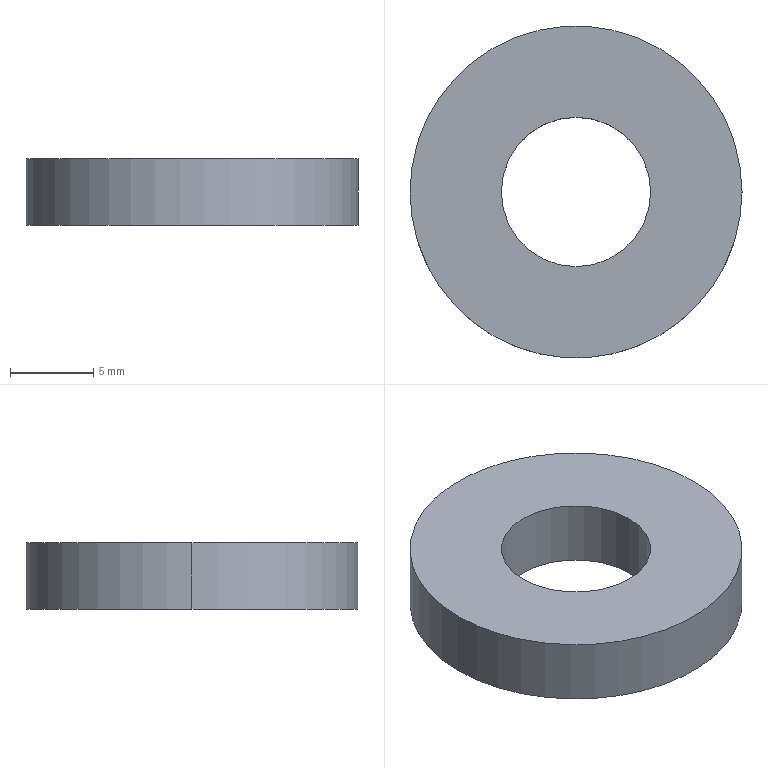Part | SolidWorks | features Extrusion 1 | 1 solid | 6 faces | box 20 x 20 x 4 mm | volume 1002 mm3 | cylinder 4 | plane 2 | commonest cylinder face diameters 9 x2 20 x2
STEP:
#1=CARTESIAN_POINT('',(-4.5,0.,4.));
#2=VERTEX_POINT('',#1);
#3=CARTESIAN_POINT('',(4.5,0.,4.));
#4=VERTEX_POINT('',#3);
#5=CARTESIAN_POINT('',(0.,0.,4.));
#6=DIRECTION('',(0.,0.,1.));
#7=DIRECTION('',(1.,0.,0.));
#8=AXIS2_PLACEMENT_3D('',#5,#6,#7);
#9=CIRCLE('',#8,4.5);
#10=EDGE_CURVE('',#2,#4,#9,.T.);
#11=ORIENTED_EDGE('',*,*,#10,.T.);
#12=CARTESIAN_POINT('',(4.5,0.,0.));
#13=VERTEX_POINT('',#12);
#14=CARTESIAN_POINT('',(4.5,0.,4.));
#15=DIRECTION('',(0.,0.,-1.));
#16=VECTOR('',#15,1000.);
#17=LINE('',#14,#16);
#18=EDGE_CURVE('',#4,#13,#17,.T.);
#19=ORIENTED_EDGE('',*,*,#18,.T.);
#20=CARTESIAN_POINT('',(-4.5,0.,0.));
#21=VERTEX_POINT('',#20);
#22=CARTESIAN_POINT('',(0.,0.,0.));
#23=DIRECTION('',(0.,0.,1.));
#24=DIRECTION('',(1.,0.,0.));
#25=AXIS2_PLACEMENT_3D('',#22,#23,#24);
#26=CIRCLE('',#25,4.5);
#27=EDGE_CURVE('',#21,#13,#26,.T.);
#28=ORIENTED_EDGE('',*,*,#27,.F.);
#29=CARTESIAN_POINT('',(-4.5,0.,4.));
#30=DIRECTION('',(0.,0.,-1.));
#31=VECTOR('',#30,1000.);
#32=LINE('',#29,#31);
#33=EDGE_CURVE('',#2,#21,#32,.T.);
#34=ORIENTED_EDGE('',*,*,#33,.F.);
#35=EDGE_LOOP('',(#11,#19,#28,#34));
#36=FACE_OUTER_BOUND('',#35,.T.);
#37=CARTESIAN_POINT('',(0.,0.,4.));
#38=DIRECTION('',(0.,0.,-1.));
#39=DIRECTION('',(-1.,0.,0.));
#40=AXIS2_PLACEMENT_3D('',#37,#38,#39);
#41=CYLINDRICAL_SURFACE('',#40,4.5);
#42=ADVANCED_FACE('',(#36),#41,.F.);
#43=CARTESIAN_POINT('',(10.,0.,4.));
#44=VERTEX_POINT('',#43);
#45=CARTESIAN_POINT('',(-10.,0.,4.));
#46=VERTEX_POINT('',#45);
#47=CARTESIAN_POINT('',(0.,0.,4.));
#48=DIRECTION('',(0.,0.,1.));
#49=DIRECTION('',(1.,0.,0.));
#50=AXIS2_PLACEMENT_3D('',#47,#48,#49);
#51=CIRCLE('',#50,10.);
#52=EDGE_CURVE('',#44,#46,#51,.T.);
#53=ORIENTED_EDGE('',*,*,#52,.F.);
#54=CARTESIAN_POINT('',(10.,0.,0.));
#55=VERTEX_POINT('',#54);
#56=CARTESIAN_POINT('',(10.,0.,4.));
#57=DIRECTION('',(0.,0.,-1.));
#58=VECTOR('',#57,1000.);
#59=LINE('',#56,#58);
#60=EDGE_CURVE('',#44,#55,#59,.T.);
#61=ORIENTED_EDGE('',*,*,#60,.T.);
#62=CARTESIAN_POINT('',(-10.,0.,0.));
#63=VERTEX_POINT('',#62);
#64=CARTESIAN_POINT('',(0.,0.,0.));
#65=DIRECTION('',(0.,0.,1.));
#66=DIRECTION('',(1.,0.,0.));
#67=AXIS2_PLACEMENT_3D('',#64,#65,#66);
#68=CIRCLE('',#67,10.);
#69=EDGE_CURVE('',#55,#63,#68,.T.);
#70=ORIENTED_EDGE('',*,*,#69,.T.);
#71=CARTESIAN_POINT('',(-10.,0.,4.));
#72=DIRECTION('',(0.,0.,-1.));
#73=VECTOR('',#72,1000.);
#74=LINE('',#71,#73);
#75=EDGE_CURVE('',#46,#63,#74,.T.);
#76=ORIENTED_EDGE('',*,*,#75,.F.);
#77=EDGE_LOOP('',(#53,#61,#70,#76));
#78=FACE_OUTER_BOUND('',#77,.T.);
#79=CARTESIAN_POINT('',(0.,0.,4.));
#80=DIRECTION('',(0.,0.,-1.));
#81=DIRECTION('',(-1.,0.,0.));
#82=AXIS2_PLACEMENT_3D('',#79,#80,#81);
#83=CYLINDRICAL_SURFACE('',#82,10.);
#84=ADVANCED_FACE('',(#78),#83,.T.);
#85=CARTESIAN_POINT('',(0.,0.,4.));
#86=DIRECTION('',(0.,0.,1.));
#87=DIRECTION('',(1.,0.,0.));
#88=AXIS2_PLACEMENT_3D('',#85,#86,#87);
#89=CIRCLE('',#88,10.);
#90=EDGE_CURVE('',#46,#44,#89,.T.);
#91=ORIENTED_EDGE('',*,*,#90,.T.);
#92=ORIENTED_EDGE('',*,*,#52,.T.);
#93=EDGE_LOOP('',(#91,#92));
#94=FACE_OUTER_BOUND('',#93,.T.);
#95=ORIENTED_EDGE('',*,*,#10,.F.);
#96=CARTESIAN_POINT('',(0.,0.,4.));
#97=DIRECTION('',(0.,0.,1.));
#98=DIRECTION('',(1.,0.,0.));
#99=AXIS2_PLACEMENT_3D('',#96,#97,#98);
#100=CIRCLE('',#99,4.5);
#101=EDGE_CURVE('',#4,#2,#100,.T.);
#102=ORIENTED_EDGE('',*,*,#101,.F.);
#103=EDGE_LOOP('',(#95,#102));
#104=FACE_BOUND('',#103,.T.);
#105=CARTESIAN_POINT('',(0.,0.,4.));
#106=DIRECTION('',(0.,0.,1.));
#107=DIRECTION('',(1.,0.,0.));
#108=AXIS2_PLACEMENT_3D('',#105,#106,#107);
#109=PLANE('',#108);
#110=ADVANCED_FACE('',(#94,#104),#109,.T.);
#111=CARTESIAN_POINT('',(0.,0.,0.));
#112=DIRECTION('',(0.,0.,1.));
#113=DIRECTION('',(1.,0.,0.));
#114=AXIS2_PLACEMENT_3D('',#111,#112,#113);
#115=CIRCLE('',#114,10.);
#116=EDGE_CURVE('',#63,#55,#115,.T.);
#117=ORIENTED_EDGE('',*,*,#116,.F.);
#118=ORIENTED_EDGE('',*,*,#69,.F.);
#119=EDGE_LOOP('',(#117,#118));
#120=FACE_OUTER_BOUND('',#119,.T.);
#121=ORIENTED_EDGE('',*,*,#27,.T.);
#122=CARTESIAN_POINT('',(0.,0.,0.));
#123=DIRECTION('',(0.,0.,1.));
#124=DIRECTION('',(1.,0.,0.));
#125=AXIS2_PLACEMENT_3D('',#122,#123,#124);
#126=CIRCLE('',#125,4.5);
#127=EDGE_CURVE('',#13,#21,#126,.T.);
#128=ORIENTED_EDGE('',*,*,#127,.T.);
#129=EDGE_LOOP('',(#121,#128));
#130=FACE_BOUND('',#129,.T.);
#131=CARTESIAN_POINT('',(0.,0.,0.));
#132=DIRECTION('',(0.,0.,1.));
#133=DIRECTION('',(1.,0.,0.));
#134=AXIS2_PLACEMENT_3D('',#131,#132,#133);
#135=PLANE('',#134);
#136=ADVANCED_FACE('',(#120,#130),#135,.F.);
#137=ORIENTED_EDGE('',*,*,#60,.F.);
#138=ORIENTED_EDGE('',*,*,#90,.F.);
#139=ORIENTED_EDGE('',*,*,#75,.T.);
#140=ORIENTED_EDGE('',*,*,#116,.T.);
#141=EDGE_LOOP('',(#137,#138,#139,#140));
#142=FACE_OUTER_BOUND('',#141,.T.);
#143=CARTESIAN_POINT('',(0.,0.,4.));
#144=DIRECTION('',(0.,0.,-1.));
#145=DIRECTION('',(-1.,0.,0.));
#146=AXIS2_PLACEMENT_3D('',#143,#144,#145);
#147=CYLINDRICAL_SURFACE('',#146,10.);
#148=ADVANCED_FACE('',(#142),#147,.T.);
#149=ORIENTED_EDGE('',*,*,#18,.F.);
#150=ORIENTED_EDGE('',*,*,#101,.T.);
#151=ORIENTED_EDGE('',*,*,#33,.T.);
#152=ORIENTED_EDGE('',*,*,#127,.F.);
#153=EDGE_LOOP('',(#149,#150,#151,#152));
#154=FACE_OUTER_BOUND('',#153,.T.);
#155=CARTESIAN_POINT('',(0.,0.,4.));
#156=DIRECTION('',(0.,0.,-1.));
#157=DIRECTION('',(-1.,0.,0.));
#158=AXIS2_PLACEMENT_3D('',#155,#156,#157);
#159=CYLINDRICAL_SURFACE('',#158,4.5);
#160=ADVANCED_FACE('',(#154),#159,.F.);
#161=CLOSED_SHELL('',(#42,#84,#110,#136,#148,#160));
#162=MANIFOLD_SOLID_BREP('',#161);
#163=CARTESIAN_POINT('',(0.,0.,0.));
#164=DIRECTION('',(0.,0.,1.));
#165=DIRECTION('',(1.,0.,0.));
#166=AXIS2_PLACEMENT_3D('',#163,#164,#165);
#167=(LENGTH_UNIT()NAMED_UNIT(*)SI_UNIT(.MILLI.,.METRE.));
#168=UNCERTAINTY_MEASURE_WITH_UNIT(LENGTH_MEASURE(0.00001),#167,'','');
#169=(NAMED_UNIT(*)PLANE_ANGLE_UNIT()SI_UNIT($,.RADIAN.));
#170=(NAMED_UNIT(*)SI_UNIT($,.STERADIAN.)SOLID_ANGLE_UNIT());
#171=(GEOMETRIC_REPRESENTATION_CONTEXT(3)GLOBAL_UNCERTAINTY_ASSIGNED_CONTEXT((#168))GLOBAL_UNIT_ASSIGNED_CONTEXT((#167,#169,#170))REPRESENTATION_CONTEXT('',''));
#172=ADVANCED_BREP_SHAPE_REPRESENTATION('',(#162,#166),#171);